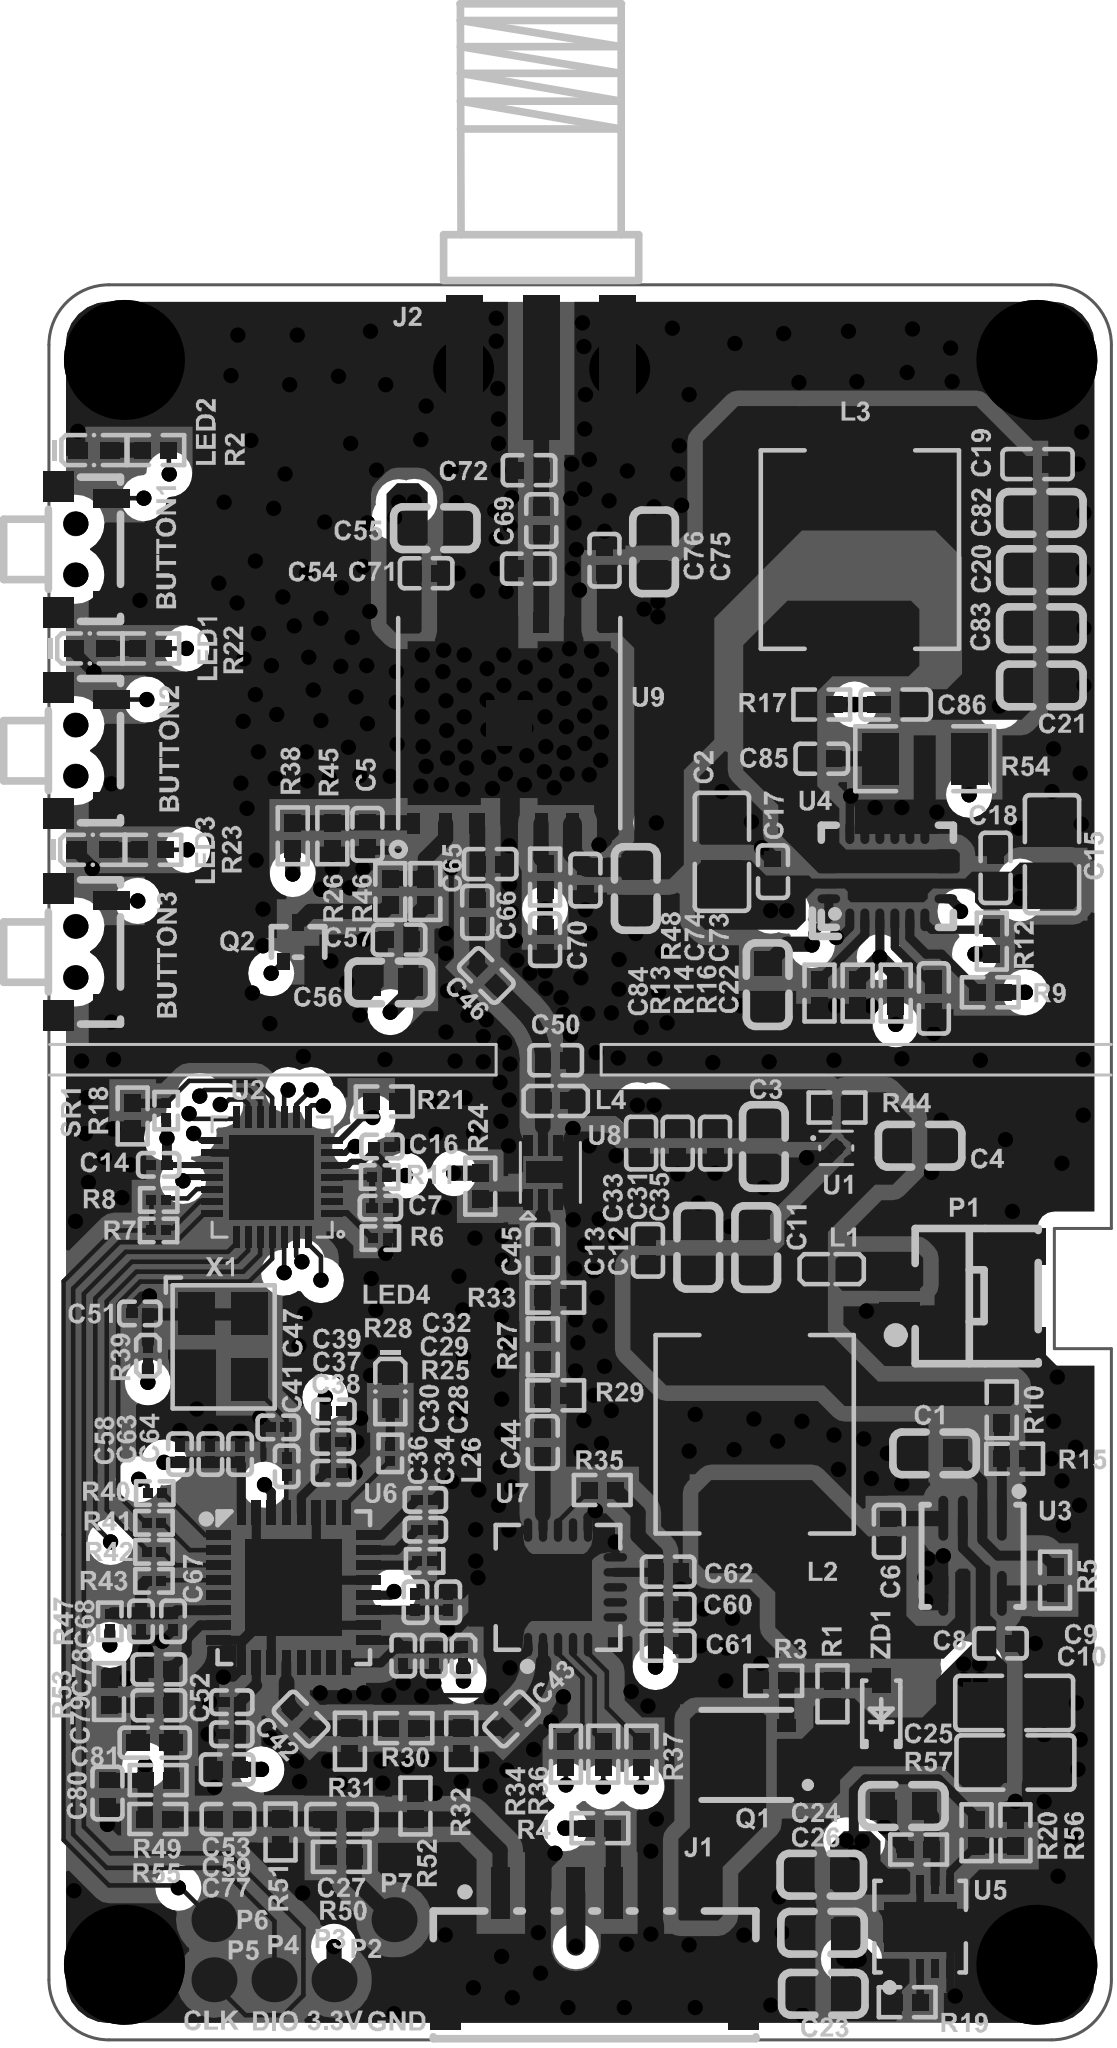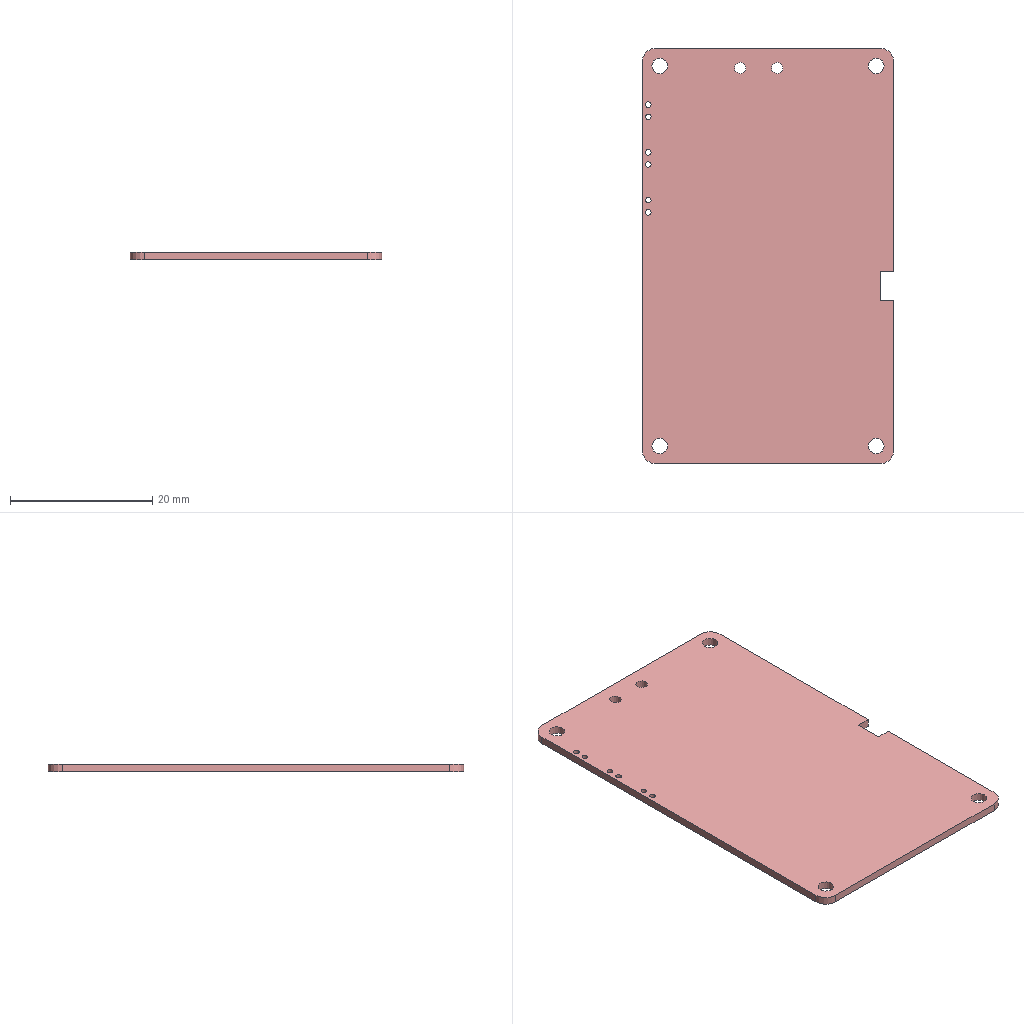Circuit board layout | Altium Designer | box 35.4 x 58.4 x 1.1 mm
Layer stack:
# Altium Designer layer stack of  (unit mm; dielectric type: 0 none, 1 core, 2 prepreg, 3 surface material)
index,name,kind,layer,copper_thickness_mm,dielectric_type,dielectric_thickness_mm,dielectric_material,dielectric_constant
0,Top Paste,other,,,,,,
1,Top Overlay,other,,,,,,
2,Top Solder,dielectric,,,3,0.0102,Solder Resist,3.5
3,Top Layer,copper,Top Layer,0.0356,,,,
4,Dielectric1,dielectric,,,1,0.32,FR-4,4.8
5,Mid-Layer 1,copper,Mid-Layer 1,0.0356,,,,
6,Dielectric2,dielectric,,,2,0.32,FR-4,4.8
7,Mid-Layer 2,copper,Mid-Layer 2,0.0356,,,,
8,Dielectric3,dielectric,,,1,0.32,FR-4,4.8
9,Bottom Layer,copper,Bottom Layer,0.0356,,,,
10,Bottom Solder,dielectric,,,3,0.0102,Solder Resist,3.5
11,Bottom Overlay,other,,,,,,
12,Bottom Paste,other,,,,,,
# drill layer pairs: low layer,high layer
drill_pair,Top Layer,Bottom Layer
Part placement:
Designator,Comment,Layer,Footprint,Center-X(mm),Center-Y(mm),Rotation
R57,33K,TopLayer,R0402,108.306,50.597,360
Q2,DULCTU3134K,TopLayer,SOT-523-3_L1.6-W0.8-P0.50-LS1.6-BR-1,87.63,80.797,270
R21,10K,TopLayer,R0402,90.5,75.489,360
U9,32A,TopLayer,AU64XX,94.666,88.077,90
P7,Pad,TopLayer,PAD,90.829,48.263,0
P6,Pad,TopLayer,PAD,84.829,48.263,0
R20,453K/1%,TopLayer,R0402,110.236,51.156,270
R19,1K,TopLayer,R0402,107.925,45.517,180
U3,AWK6943,TopLayer,QFN-8_L3.0-W3.0-P0.65-BL,110.104,60.37,180
L2,SL0624-100M,TopLayer,IND-SMD_L7.1-W6.6,102.845,64.414,90
C10,10uF,TopLayer,C0805,111.531,53.492,360
C9,10uF,TopLayer,C0805,111.49,55.474,360
R5,100K,TopLayer,R0402,112.852,59.563,270
R15,24.9K,TopLayer,R0402,111.506,63.602,360
R10,107K,TopLayer,R0402,111.074,65.227,270
L1,MPZ1005S121CT000,TopLayer,L0402,105.41,69.901,180
C1,1uf,TopLayer,C0603,108.839,63.779,180
C13,100nf,TopLayer,C0402,99.289,70.536,90
C12,22uF,TopLayer,C0603,100.965,70.637,90
C11,22uF,TopLayer,C0603,102.895,70.626,90
C8,100nf,TopLayer,C0402,111.033,57.455,360
C6,0.1uF,TopLayer,C0402,107.315,61.189,270
C3,1uF,TopLayer,C0603,103.149,73.99,270
C4,1uF,TopLayer,C0603,108.356,74.016,360
C5,0.1uF,TopLayer,C0402,89.941,84.379,90
C7,100nf,TopLayer,C0201,90.373,71.958,180
C14,100nf,TopLayer,C0201,82.987,73.381,180
C16,100nf,TopLayer,C0201,90.424,73.99,360
C23,4.7uF,TopLayer,C0603,105.131,45.796,360
C24,4.7uF,TopLayer,C0603,105.08,49.759,360
C25,4.7uF,TopLayer,C0603,107.798,52.045,360
C26,22uF,TopLayer,C0603,105.105,47.828,180
C28,0.1uF,TopLayer,C0201,92.634,58.826,270
C29,0.1uF,TopLayer,C0201,91.872,61.239,360
C30,1NF,TopLayer,C0201,91.542,58.826,90
C31,1UF,TopLayer,C0402,100.279,74.103,90
C32,1NF,TopLayer,C0201,91.872,62.23,180
C33,100nf,TopLayer,C0402,99.06,74.103,90
C34,0.1uF,TopLayer,C0201,92.151,57.048,90
C35,10PF   50V,TopLayer,C0402,101.524,74.103,270
C36,1NF,TopLayer,C0201,91.135,57.048,270
C37,0.1uF,TopLayer,C0201,88.798,64.16,180
C38,1NF,TopLayer,C0201,88.81,63.135,360
C39,0.1uF,TopLayer,C0201,88.824,65.176,180
C41,1NF,TopLayer,C0201,87.249,63.348,90
C42,10PF,TopLayer,C0402,87.732,54.94,315
C43,10PF,TopLayer,C0402,94.742,54.94,45
C44,10PF,TopLayer,C0402,95.783,64.147,90
C45,10PF,TopLayer,C0402,95.783,70.51,90
C46,10PF,TopLayer,C0402,93.904,79.68,135
C47,1NF,TopLayer,C0201,86.97,64.643,180
C50,NC,TopLayer,C0402,96.215,76.86,360
C51,1NF,TopLayer,C0201,82.356,68.436,360
C52,100PF,TopLayer,C0201,85.42,55.499,180
C53,0.1uF,TopLayer,C0201,85.42,54.432,360
C58,1NF,TopLayer,C0201,83.693,63.754,270
C59,10uF,TopLayer,C0402,85.268,53.264,360
C60,1NF,TopLayer,C0402,99.961,58.598,180
C61,100nf,TopLayer,C0402,99.961,57.379,180
C62,1UF,TopLayer,C0402,99.961,59.842,180
C63,1NF,TopLayer,C0201,84.709,63.754,270
C64,1NF,TopLayer,C0201,85.7,63.754,90
C67,1NF,TopLayer,C0201,83.464,58.191,270
C68,0.1uF,TopLayer,C0201,82.398,58.191,90
C77,4.7UF,TopLayer,C0402,85.293,51.613,180
C78,4.7UF,TopLayer,C0402,82.993,56.591,180
C79,22UF,TopLayer,C0402,82.993,55.397,360
C80,2PF,TopLayer,C0402,81.28,52.476,90
R1,50K,TopLayer,R0402,105.435,55.778,270
R2,3.3K,TopLayer,R0402,82.891,97.163,180
R3,100K,TopLayer,R0402,103.48,56.21,360
R4,1K,TopLayer,R0402,97.688,51.308,180
R6,10K,TopLayer,R0201,90.373,70.942,180
R7,22R,TopLayer,R0201,82.982,71.196,180
R8,22R,TopLayer,R0201,82.987,72.212,180
R11,10K,TopLayer,R0201,90.348,72.974,360
R18,10K,TopLayer,R0201,83.236,75.184,90
R22,3.3K,TopLayer,R0402,82.723,90.563,180
R23,3.3K,TopLayer,R0402,82.793,83.863,180
R24,3.9K,TopLayer,R0402,93.701,72.669,270
R25,4.7K,TopLayer,R0201,91.846,60.198,180
R27,30R,TopLayer,R0402,95.783,67.322,90
R28,4.7K,TopLayer,R0201,90.703,63.779,270
R29,180R,TopLayer,R0402,96.215,65.71,360
R30,18R,TopLayer,R0402,91.159,54.635,0
R31,300R,TopLayer,R0402,89.357,54.204,270
R32,300R,TopLayer,R0402,93.066,54.204,270
R33,180R,TopLayer,R0402,96.215,68.961,360
R34,0R,TopLayer,R0402,96.555,53.769,270
R35,0R,TopLayer,R0402,97.765,62.56,360
R36,0R,TopLayer,R0402,97.799,53.769,270
R37,0R,TopLayer,R0402,99.069,53.769,270
R40,0R,TopLayer,R0201,82.855,62.459,180
R41,0R,TopLayer,R0201,82.829,61.468,180
R42,0R,TopLayer,R0201,82.829,60.503,180
R43,0R,TopLayer,R0201,82.829,59.538,180
R47,0R,TopLayer,R0201,81.356,58.191,270
R49,20K,TopLayer,R0402,82.967,52.908,180
R50,270R,TopLayer,R0402,89.068,50.353,360
R51,10R,TopLayer,R0402,87.046,51.181,270
R52,91R,TopLayer,R0402,91.542,52.045,90
R53,22R,TopLayer,R0402,81.331,55.855,90
SR1,SDNT1005X103F3380FTF,TopLayer,R0402,82.118,75.006,270
J1,WAFER-GH1. 25-6PWB,TopLayer,SMD_6P-P1.25_XUNPU_WAFER-GH1.25-6PWB,97.51,47.574,360
BUTTON1,TS24CA250GF013,TopLayer,SW-SMD_L4.7-W3.5-P3.35-EH,80.529,93.863,360
BUTTON2,TS24CA250GF013,TopLayer,SW-SMD_L4.7-W3.5-P3.35-EH,80.529,87.163,360
BUTTON3,TS24CA250GF013,TopLayer,SW-SMD_L4.7-W3.5-P3.35-EH,80.529,80.463,360
U5,DU3042,TopLayer,WSON-10_L3.0-W3.0-P0.50-BL-EP,108.356,48.031,360
U1,TPS7A2050PDQNR,TopLayer,X2SON-4_L1.0-W1.0-P0.65-TL-EP,105.562,73.939,0
U2,GD32E230G8U6,TopLayer,QFN-28_L4.0-W4.0-P0.40-BL-EP2.8,86.766,72.974,90
LED1,LED,TopLayer,LED0402,80.691,90.563,360
LED2,LED,TopLayer,LED0402,80.829,97.163,360
LED3,LED,TopLayer,LED0402,80.791,83.863,360
LED4,LED,TopLayer,LED0402,90.703,65.837,270
SCREW2,MARK_4,TopLayer,M2,81.829,100.163,90
SCREW3,MARK_4,TopLayer,M2,112.229,46.763,90
SCREW4,MARK_4,TopLayer,M2,112.229,100.163,90
P2,Pad,TopLayer,PAD,90.829,46.263,0
P3,Pad,TopLayer,PAD,88.829,46.263,0
P4,Pad,TopLayer,PAD,86.829,46.263,0
P5,Pad,TopLayer,PAD,84.829,46.263,0
X1,OT322525MJBA4SL,TopLayer,SMD3225,85.129,67.343,270
U7,ARW621A,TopLayer,QFN-20_L4.0-W4.0-P0.50-TL-EP2.2,96.291,59.321,90
L4,33nH,TopLayer,L0402,96.215,75.514,360
L26,BLM03PX800SN1D,TopLayer,L0201,93.142,57.048,90
R39,BLM03PX800SN1D,TopLayer,L0201,82.626,67.031,90
P1,WAFER-SHB1.0-2PWB,TopLayer,SMD_2P-WAFER-SHB1.0-2PWB,109.541,69.013,90
ZD1,BZT52C15S,TopLayer,SOD-323_L1.7-W1.3-LS2.6-RD,107.061,55.093,90
Q1,CJAE10P06,TopLayer,DFN-8_L3.0-W3.0-P0.65-BL_G48N03D3,102.54,53.746,90
U6,GX1288FL,TopLayer,QFN-32_L5.0-W5.0-P0.50,87.488,59.309,360
U8,CBG9092,TopLayer,CBG9092,96.037,73.127,90
C27,150PF,TopLayer,C0402,89.078,51.613,180
C81,22uF,TopLayer,C0402,82.855,54.153,360
C54,10PF,TopLayer,C0402,91.897,93.066,360
C55,4.7UF,TopLayer,C0603,92.202,94.564,360
C56,4.7UF,TopLayer,C0603,90.69,79.451,360
C57,10PF,TopLayer,C0402,90.995,80.874,360
C65,NC,TopLayer,C0402,94.031,83.388,360
C66,10PF,TopLayer,C0402,93.599,81.788,270
C69,10PF,TopLayer,C0402,95.733,94.818,90
C70,2.2NF,TopLayer,C0402,95.86,80.874,90
C71,NC,TopLayer,C0402,95.301,93.218,360
C72,NC,TopLayer,C0402,95.326,96.495,360
C73,4.7uF,TopLayer,C0603,98.882,82.575,270
C74,10PF,TopLayer,C0402,97.206,82.855,270
C75,4.7UF,TopLayer,C0603,99.492,93.777,90
C76,10PF,TopLayer,C0402,97.841,93.497,90
R38,0R,TopLayer,R0402,87.452,84.328,90
R45,1MR,TopLayer,R0402,88.773,84.328,270
R46,0R,TopLayer,R0402,91.872,82.474,90
R48,,TopLayer,R0402,95.86,82.956,90
SCREW1,MARK_4,TopLayer,M2,81.829,46.763,90
J2,SMA-50KE-3,TopLayer,SMA-FP-945G,95.729,99.888,90
R26,1K,TopLayer,R0402,90.703,82.474,270
R55,2K,TopLayer,R0402,82.956,51.613,360
R56,49.9K/1%,TopLayer,R0402,111.531,51.156,90
R54,4.7R,TopLayer,R1206,108.509,86.893,360
C18,100nf,TopLayer,C0402,110.871,83.261,90
C15,10uF,TopLayer,C0805,112.751,83.718,90
R17,845K,TopLayer,R0402,105.08,88.697,360
C86,390pF,TopLayer,C0402,107.544,88.697,180
C17,100nf,TopLayer,C0402,103.454,83.134,90
C85,0.1uF,TopLayer,C0402,105.08,86.893,180
L3,SL0624-100M,TopLayer,IND-SMD_L7.1-W6.6,106.35,93.853,90
R9,499K,TopLayer,R0402,110.693,79.121,360
R12,100K,TopLayer,R0402,110.744,80.823,270
R13,100K,TopLayer,R0402,105.004,79.096,270
R14,10.1K,TopLayer,R0402,106.274,79.095,270
R16,60K,TopLayer,R0402,107.544,79.095,90
U4,MP4470GL-Z,TopLayer,QFN-20_L4.0-W3.0_MP9447GL,107.264,82.982,90
C20,22uF,TopLayer,C0603,112.395,93.167,360
C21,22uF,TopLayer,C0603,112.395,89.332,360
C22,33nF,TopLayer,C0402,108.814,78.918,90
C82,22uF,TopLayer,C0603,112.395,95.072,360
C83,22uF,TopLayer,C0603,112.395,91.237,360
C84,1uf,TopLayer,C0603,103.276,79.375,270
C2,10uF,TopLayer,C0805,101.752,83.795,90
C19,0.1uF,TopLayer,C0402,112.268,96.698,180
R44,NC,TopLayer,R0402,105.588,75.286,180
Pad and via stacks:
# Altium Designer via and pad stacks of  (unit mm). Each distinct definition once, with the count of objects using it.
# via: kind,start_layer,end_layer,hole_mm,diameter_mm,mode(0 simple;1 top-mid-bottom;2 full stack),diameter_per_layer,count,example_net
# pad: kind,layer,hole_mm,hole_type(0 round;1 square;2 slot),plating,top_size,top_shape(1 round;2 rect;3 octagon;9 rounded rect),mid_size,bottom_size,mode,footprint,size_per_layer,count,example
pad,Top Layer,0,0,plated,0.5657x0.54,2,0.5657x0.54,0.5657x0.54,0,R0402,,88,R57.1
pad,Top Layer,0,0,plated,0.5334x0.4064,2,0.5334x0.4064,0.5334x0.4064,0,SOT-523-3_L1.6-W0.8-P0.50-LS1.6-BR-1,,2,Q2.1
pad,Top Layer,0,0,plated,0.5334x0.4,2,0.5334x0.4,0.5334x0.4,0,SOT-523-3_L1.6-W0.8-P0.50-LS1.6-BR-1,,1,Q2.3
pad,Top Layer,0,0,plated,4.8x1.2,2,4.8x1.2,4.8x1.2,0,SMA-FP-945G,,3,J2.1
pad,Top Layer,0,0,plated,0.3x0.67,2,0.3x0.67,0.3x0.67,0,CBG9092,,8,U8.1
pad,Top Layer,0,0,plated,0.7x1.6,2,0.7x1.6,0.7x1.6,0,CBG9092,,1,U8.9
pad,Top Layer,0,0,plated,3.2x3.2,2,3.2x3.2,3.2x3.2,0,QFN-32_L5.0-W5.0-P0.50,,1,U6.33
pad,Top Layer,0,0,plated,0.3x0.8,2,0.3x0.8,0.3x0.8,0,QFN-32_L5.0-W5.0-P0.50,,32,U6.32
pad,Top Layer,0,0,plated,2.6x2,2,2.6x2,2.6x2,0,DFN-8_L3.0-W3.0-P0.65-BL_G48N03D3,,1,Q1.9
pad,Top Layer,0,0,plated,0.4x0.6,2,0.4x0.6,0.4x0.6,0,DFN-8_L3.0-W3.0-P0.65-BL_G48N03D3,,8,Q1.5
pad,Top Layer,0,0,plated,0.63x0.83,2,0.63x0.83,0.63x0.83,0,SOD-323_L1.7-W1.3-LS2.6-RD,,2,ZD1.1
pad,Top Layer,0,0,plated,1.2x2.22,2,1.2x2.22,1.2x2.22,0,SMD_2P-WAFER-SHB1.0-2PWB,,2,P1.4
pad,Top Layer,0,0,plated,0.6x1.35,2,0.6x1.35,0.6x1.35,0,SMD_2P-WAFER-SHB1.0-2PWB,,2,P1.2
pad,Top Layer,0,0,plated,0.3684x0.324,2,0.3684x0.324,0.3684x0.324,0,L0201,,4,L26.1
pad,Top Layer,0,0,plated,2.2x2.2,2,2.2x2.2,2.2x2.2,0,QFN-20_L4.0-W4.0-P0.50-TL-EP2.2,,1,U7.21
pad,Top Layer,0,0,plated,0.28x0.79,1,0.28x0.79,0.28x0.79,0,QFN-20_L4.0-W4.0-P0.50-TL-EP2.2,,10,U7.20
pad,Top Layer,0,0,plated,0.79x0.28,1,0.79x0.28,0.79x0.28,0,QFN-20_L4.0-W4.0-P0.50-TL-EP2.2,,10,U7.15
pad,Top Layer,0,0,plated,1.4x1.2,2,1.4x1.2,1.4x1.2,0,SMD3225,,4,X1.4
pad,Top Layer,0,0,plated,0.6365x0.54,2,0.6365x0.54,0.6365x0.54,0,LED0402,,8,LED1.1
pad,Top Layer,0,0,plated,0.2x0.7,2,0.2x0.7,0.2x0.7,0,QFN-28_L4.0-W4.0-P0.40-BL-EP2.8,,14,U2.4
pad,Top Layer,0,0,plated,0.7x0.2,2,0.7x0.2,0.7x0.2,0,QFN-28_L4.0-W4.0-P0.40-BL-EP2.8,,14,U2.8
pad,Top Layer,0,0,plated,2.8x2.8,2,2.8x2.8,2.8x2.8,0,QFN-28_L4.0-W4.0-P0.40-BL-EP2.8,,1,U2.29
pad,Top Layer,0,0,plated,0.4801x0.4801,2,0.4801x0.4801,0.4801x0.4801,0,X2SON-4_L1.0-W1.0-P0.65-TL-EP,,1,U1.5
pad,Top Layer,0,0,plated,0.1247x0.1247,1,0.1247x0.1247,0.1247x0.1247,0,X2SON-4_L1.0-W1.0-P0.65-TL-EP,,4,U1.4
pad,Top Layer,0,0,plated,0.6x1.2,2,0.6x1.2,0.6x1.2,0,SW-SMD_L4.7-W3.5-P3.35-EH,,6,BUTTON1.2
pad,Top Layer,0,0,plated,1x1,2,1x1,1x1,0,SW-SMD_L4.7-W3.5-P3.35-EH,,6,BUTTON1.3
pad,Top Layer,0,0,plated,1x2.8,2,1x2.8,1x2.8,0,SMD_6P-P1.25_XUNPU_WAFER-GH1.25-6PWB,,2,J1.8
pad,Top Layer,0,0,plated,0.6x1.7,2,0.6x1.7,0.6x1.7,0,SMD_6P-P1.25_XUNPU_WAFER-GH1.25-6PWB,,6,J1.4
pad,Top Layer,0,0,plated,0.3031x0.324,2,0.3031x0.324,0.3031x0.324,0,R0201,,24,R6.2
pad,Top Layer,0,0,plated,0.3684x0.324,2,0.3684x0.324,0.3684x0.324,0,C0201,,44,C7.2
pad,Top Layer,0,0,plated,0.8x0.9,2,0.8x0.9,0.8x0.9,0,C0603,,36,C1.1
pad,Top Layer,0,0,plated,0.54x0.54,2,0.54x0.54,0.54x0.54,0,L0402,,4,L1.2
pad,Top Layer,0,0,plated,1.41x1.35,2,1.41x1.35,1.41x1.35,0,C0805,,8,C10.1
pad,Top Layer,0,0,plated,2.15x3.32,2,2.15x3.32,2.15x3.32,0,IND-SMD_L7.1-W6.6,,4,L2.1
pad,Top Layer,0,0,plated,0.33x1.5,1,0.33x1.5,0.33x1.5,0,QFN-8_L3.0-W3.0-P0.65-BL,,8,U3.1
pad,Top Layer,0,0,plated,1.5x1.5,1,1.5x1.5,1.5x1.5,0,PAD,,6,P7.1
pad,Top Layer,0,0,plated,0.5x0.54,2,0.5x0.54,0.5x0.54,0,C0402,,66,C6.1
pad,Top Layer,0,0,plated,0.7901x0.54,2,0.7901x0.54,0.7901x0.54,0,C0402,,12,C27.2
pad,Top Layer,0,0,plated,2.4x1.65,2,2.4x1.65,2.4x1.65,0,WSON-10_L3.0-W3.0-P0.50-BL-EP,,1,U5.11
pad,Top Layer,0,0,plated,0.25x0.6,2,0.25x0.6,0.25x0.6,0,WSON-10_L3.0-W3.0-P0.50-BL-EP,,10,U5.1
pad,Top Layer,0,0,plated,1.208x1.701,2,1.208x1.701,1.208x1.701,0,R1206,,2,R54.1
pad,Top Layer,0,0,plated,0.76x0.3,1,0.76x0.3,0.76x0.3,0,QFN-20_L4.0-W3.0_MP9447GL,,20,U4.20
pad,Top Layer,0,0,plated,0.5x0.4,2,0.5x0.4,0.5x0.4,0,QFN-20_L4.0-W3.0_MP9447GL,,5,U4.21
pad,Top Layer,0,0,plated,0.675x0.4,2,0.675x0.4,0.675x0.4,0,AU64XX,,12,U9.1
pad,Top Layer,0,0,plated,0.675x0.4999,2,0.675x0.4999,0.675x0.4999,0,AU64XX,,2,U9.3
pad,Top Layer,0,0,plated,1.524x1.524,2,1.524x1.524,1.524x1.524,0,AU64XX,,1,U9.15
pad,Multi-Layer,1.6,0,plated,2x2,1,2x2,2x2,0,SMA-FP-945G,,2,J2.2
pad,Multi-Layer,2.2,0,plated,4x4,1,4x4,4x4,0,M2,,4,SCREW2.1
pad,Multi-Layer,0.8,0,unplated,0.8x0.8,1,0.8x0.8,0.8x0.8,0,SW-SMD_L4.7-W3.5-P3.35-EH,,6,BUTTON1.0
pad,Bottom Layer,0,0,plated,4.8x1.2,2,4.8x1.2,4.8x1.2,0,SMA-FP-945G,,2,J2.2
via,Top Layer,Bottom Layer,0.3048,0.508,0,,554,GND
Copper pours:
name,layer,net,type(0 solid;1 hatched;2 none)
Bottom Layer-No Net,Top Layer,PA_5.5V,0
Bottom Layer-No Net,Top Layer,NetC85_2,0
Bottom Layer-No Net,Top Layer,POWER-IN,0
Bottom Layer-No Net,Top Layer,3.3V,0
Bottom Layer-No Net,Top Layer,VCC_5V,0
Bottom Layer-No Net,Top Layer,POWER-IN,0
Bottom Layer-No Net,Top Layer,PA_5.5V,0
Bottom Layer-No Net,Top Layer,GND,0
Bottom Layer-No Net,Top Layer,VCC_5V3,0
Bottom Layer-No Net,Top Layer,VCC_5V,0
Bottom Layer-No Net,Top Layer,+5V-FAN,0
Bottom Layer-No Net,Top Layer,NetC6_2,0
Bottom Layer-No Net,Top Layer,NetJ1_6,0
Bottom Layer-No Net,Mid-Layer 2,POWER-IN,0
Bottom Layer-No Net,Mid-Layer 2,PA_5.5V,0
Bottom Layer-No Net,Mid-Layer 2,GND,0
Bottom Layer-No Net,Mid-Layer 2,VCC_5V,0
Bottom Layer-No Net,Mid-Layer 2,VCC_5V,0
Bottom Layer-No Net,Mid-Layer 2,3.3V,0
Bottom Layer-No Net,Bottom Layer,GND,0
Bottom Layer-No Net,Mid-Layer 1,GND,0
Design rules, without the lines most boards share:
# Altium Designer design rules of  (exported by Altium Designer, unit mm)
# columns: name | kind | enabled | priority | scope1 | scope2 | descriptor | typed fields (field=value)
Clearance_5 | 0 | enabled | 1 | INPOLYGON | All | Clearance Constraint (Gap=6mil) (INPOLYGON),(All) | gap=0.1524
Clearance | 0 | enabled | 2 | All | All | Clearance Constraint (Gap=6mil) (All),(All) | gap=0.1524
PlaneConnect | 6 | enabled | 1 | All | All | Power Plane Connect Rule(Direct Connect )(Expansion=20mil) (Conductor Width=10mil) (Air Gap=10mil) (Entries=4) (All) | relief_conductor_width=0.254 relief_entries=4 relief_expansion=0.508
PlaneClearance | 12 | enabled | 1 | All | All | Power Plane Clearance (Clearance =6mil) (All) | clearance=0.1524
PolygonConnect | 20 | enabled | 1 | All | All | Polygon Connect Rule(Direct Connect )(Conductor Width=10mil) (Relief Angle=90 Angle) (Entries=4) (Air Gap Width=10mil) (All),(All) | connect_style(0=relief,1=direct,2=none)=1 relief_conductor_width=0.254 relief_entries=4
Width | 2 | enabled | 1 | All | All | Width Constraint (Min=6mil) (Max=100mil) (Preferred=6mil) (All) |
RoutingVias | 11 | enabled | 1 | All | All | Routing Via (MinHoleWidth=12mil) (MaxHoleWidth=12mil) (PreferredHoleWidth=12mil) (MinWidth=20mil) (MaxWidth=20mil) (PreferedWidth=20mil) (All) | via_min_hole=0.3048 via_max_hole=0.3048 via_preferred_diameter=0.508 via_preferred_hole=0.3048
SolderMaskExpansion | 13 | enabled | 1 | All | All | Solder Mask Expansion (Expansion =4mil) (All) | expansion=0.1016
HoleSize | 42 | enabled | 1 | All | All | Hole Size Constraint (Min=1mil) (Max=500mil) (All) |
DiffPairsRouting | 51 | enabled | 1 | All | All | Differential Pairs Uncoupled Length using the Gap Constraints (Min=6mil) (Max=6mil) (Prefered=6mil)  and Width Constraints (Min=15mil) (Max=15mil) (Prefered=15mil) (All) |
HoleToHoleClearance | 52 | enabled | 1 | All | All | Hole To Hole Clearance (Gap=0mil) (All),(All) | gap=0
MinimumSolderMaskSliver | 53 | enabled | 1 | All | All | Minimum Solder Mask Sliver (Gap=0mil) (All),(All) |
SilkscreenOverComponentPads | 54 | enabled | 1 | IsPad | All | Silk To Solder Mask (Clearance=0mil) (IsPad),(All) |
SilkToSilkClearance | 55 | enabled | 1 | All | All | Silk to Silk (Clearance=0mil) (All),(All) |
Classes set for this board:
# Altium Designer classes of  (member kind: 0 net, 1 component, 2 from-to, 3 pad, 4 layer, 5 differential pair, 6 design channel, 7 polygon, 8 structure, 9 xSignal)
# columns: class name | member kind | superclass | members
3.3G_GX1288FL_5W | 1 | no | BUTTON1; BUTTON2; BUTTON3; C3; C4; C5; C6; C7; C8; C9; C10; C11; C12; C13; C14; C2; C16; C17; C18; C19; C20; C21; C22; C23; C24; C25; C26; C27; C28; C29; C30; C31; C32; C33; C34; C35; C36; C37; C38; C39; C41; C42; C43; C44; C45; C46; C47; C50; C51; C52; C53; C54; C55; C56; C57; C58; C59; C60; C61; C62; C63; C64; C65; C66; C67; C68; C69; C70; C71; C72; C73; C74; C75; C76; C77; C78; C79; C80; J1; J2; L1; L2; L3; L4; LED1; LED2; LED3; LED4; P1; P2; P3; P4; P5; Q1; R1; R3; R4; R5; R6; R7; R8; R9; R10; R11; R12; R13; R14; R15; R16; R17; R18; R19; R22; R25; R26; R28; R30; R31; R32; R35; R39; R40; R41; R42; R43; R45; R46; R47; R48; R49; R50; R51; R52; R5; R?; R?; R?; R?; R?; R?; R?; R?; R?; R?; SCREW1; SCREW2; SCREW3; SCREW4; SR1; U1; U2; U3; U4; U5; U6; U7; U8; U9; X1; ZD1; R1; R3; R4; R6; R7; R8; R11; R18; R22; R25; R28; R30; R31; R32; R35; R40; R41; R42; R43; R47; R49; R50; R51; R52; R?; R?; R?; R?; R?; R?; R?; R?; R?; R?; R?; SR1; C3; C4; C5; C7; C14; C16; C23; C24; C25; C26; C28; C29; C30; C31; C32; C33; C34; C35; C36; C37; C38; C39; C41; C42; C43; C44; C45; C46; C47; C50; C51; C52; C53; C58; C59; C60; C61; C62; C63; C64; C67; C68; C77; C78; C79; C80; R1; R2; R3; R4; R6; R7; R8; R11; R18; R22; R23; R24; R25; R27; R28; R29; R30; R31; R32; R33; R34; R35; R36; R37; R40; R41; R42; R43; R47; R49; R50; R51; R52; R53; SR1; J1; BUTTON1; BUTTON2; BUTTON3; U5; U1; U2; LED1; LED2; LED3; LED4; SCREW2; SCREW3; SCREW4; P2; P3; P4; P5; X1; U7; L4; L26; R39; P1; ZD1; Q1; U6; U8; C6; C8; C11; C12; C13; C1; L1; R10; R15; R?; C9; C10; L2; U3; C17; C18; C85; L3; R9; R12; R13; R14; R16; U4; C2; C20; C21; C22; C27; C81; C82; C83; C84; C15; C19; C54; C55; C56; C57; C65; C66; C69; C70; C71; C72; C73; C74; C75; C76; R38; R45; R46; R48; SCREW1; J2; U9; C86; R17; R19; R20; P6; P7; U9; R21; R26; R44; R54; R55; R56; R54; C18; C15; R17; C86; C17; C85; L3; R9; R12; R13; R14; R16; U4; C20; C21; C22; C82; C83; C84; C2; C19; R44; Q2; R57;